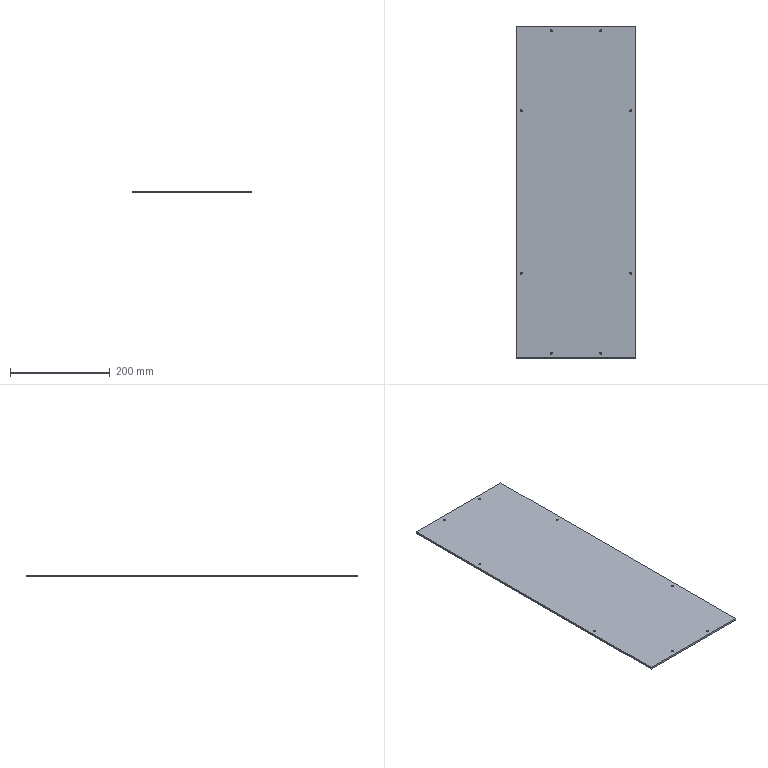Part | SolidWorks | features HoleWzd 2, MirrorPattern 2, Extrusion 1 | 1 solid | 22 faces | box 240 x 666 x 4 mm | volume 638958 mm3 | cylinder 16 | plane 6 | commonest cylinder face diameters 4 x16
STEP:
#1=CARTESIAN_POINT('',(-108.,163.,2.));
#2=VERTEX_POINT('',#1);
#3=CARTESIAN_POINT('',(-112.,163.,2.));
#4=VERTEX_POINT('',#3);
#5=CARTESIAN_POINT('',(-110.,163.,2.));
#6=DIRECTION('',(0.,0.,-1.));
#7=DIRECTION('',(-1.,0.,0.));
#8=AXIS2_PLACEMENT_3D('',#5,#6,#7);
#9=CIRCLE('',#8,2.);
#10=EDGE_CURVE('',#2,#4,#9,.T.);
#11=ORIENTED_EDGE('',*,*,#10,.F.);
#12=CARTESIAN_POINT('',(-108.,163.,-2.));
#13=VERTEX_POINT('',#12);
#14=CARTESIAN_POINT('',(-108.,163.,-2.));
#15=DIRECTION('',(0.,0.,-1.));
#16=VECTOR('',#15,1000.);
#17=LINE('',#14,#16);
#18=EDGE_CURVE('',#2,#13,#17,.T.);
#19=ORIENTED_EDGE('',*,*,#18,.T.);
#20=CARTESIAN_POINT('',(-112.,163.,-2.));
#21=VERTEX_POINT('',#20);
#22=CARTESIAN_POINT('',(-110.,163.,-2.));
#23=DIRECTION('',(0.,0.,-1.));
#24=DIRECTION('',(-1.,0.,0.));
#25=AXIS2_PLACEMENT_3D('',#22,#23,#24);
#26=CIRCLE('',#25,2.);
#27=EDGE_CURVE('',#13,#21,#26,.T.);
#28=ORIENTED_EDGE('',*,*,#27,.T.);
#29=CARTESIAN_POINT('',(-112.,163.,-2.));
#30=DIRECTION('',(0.,0.,-1.));
#31=VECTOR('',#30,1000.);
#32=LINE('',#29,#31);
#33=EDGE_CURVE('',#4,#21,#32,.T.);
#34=ORIENTED_EDGE('',*,*,#33,.F.);
#35=EDGE_LOOP('',(#11,#19,#28,#34));
#36=FACE_OUTER_BOUND('',#35,.T.);
#37=CARTESIAN_POINT('',(-110.,163.,-2.));
#38=DIRECTION('',(0.,0.,-1.));
#39=DIRECTION('',(-1.,0.,0.));
#40=AXIS2_PLACEMENT_3D('',#37,#38,#39);
#41=CYLINDRICAL_SURFACE('',#40,2.);
#42=ADVANCED_FACE('',(#36),#41,.F.);
#43=CARTESIAN_POINT('',(-108.,-163.,2.));
#44=VERTEX_POINT('',#43);
#45=CARTESIAN_POINT('',(-112.,-163.,2.));
#46=VERTEX_POINT('',#45);
#47=CARTESIAN_POINT('',(-110.,-163.,2.));
#48=DIRECTION('',(0.,0.,-1.));
#49=DIRECTION('',(-1.,0.,0.));
#50=AXIS2_PLACEMENT_3D('',#47,#48,#49);
#51=CIRCLE('',#50,2.);
#52=EDGE_CURVE('',#44,#46,#51,.T.);
#53=ORIENTED_EDGE('',*,*,#52,.F.);
#54=CARTESIAN_POINT('',(-108.,-163.,-2.));
#55=VERTEX_POINT('',#54);
#56=CARTESIAN_POINT('',(-108.,-163.,-2.));
#57=DIRECTION('',(0.,0.,-1.));
#58=VECTOR('',#57,1000.);
#59=LINE('',#56,#58);
#60=EDGE_CURVE('',#44,#55,#59,.T.);
#61=ORIENTED_EDGE('',*,*,#60,.T.);
#62=CARTESIAN_POINT('',(-112.,-163.,-2.));
#63=VERTEX_POINT('',#62);
#64=CARTESIAN_POINT('',(-110.,-163.,-2.));
#65=DIRECTION('',(0.,0.,-1.));
#66=DIRECTION('',(-1.,0.,0.));
#67=AXIS2_PLACEMENT_3D('',#64,#65,#66);
#68=CIRCLE('',#67,2.);
#69=EDGE_CURVE('',#55,#63,#68,.T.);
#70=ORIENTED_EDGE('',*,*,#69,.T.);
#71=CARTESIAN_POINT('',(-112.,-163.,-2.));
#72=DIRECTION('',(0.,0.,-1.));
#73=VECTOR('',#72,1000.);
#74=LINE('',#71,#73);
#75=EDGE_CURVE('',#46,#63,#74,.T.);
#76=ORIENTED_EDGE('',*,*,#75,.F.);
#77=EDGE_LOOP('',(#53,#61,#70,#76));
#78=FACE_OUTER_BOUND('',#77,.T.);
#79=CARTESIAN_POINT('',(-110.,-163.,-2.));
#80=DIRECTION('',(0.,0.,-1.));
#81=DIRECTION('',(-1.,0.,0.));
#82=AXIS2_PLACEMENT_3D('',#79,#80,#81);
#83=CYLINDRICAL_SURFACE('',#82,2.);
#84=ADVANCED_FACE('',(#78),#83,.F.);
#85=CARTESIAN_POINT('',(52.,-323.,2.));
#86=VERTEX_POINT('',#85);
#87=CARTESIAN_POINT('',(48.,-323.,2.));
#88=VERTEX_POINT('',#87);
#89=CARTESIAN_POINT('',(50.,-323.,2.));
#90=DIRECTION('',(0.,0.,-1.));
#91=DIRECTION('',(-1.,0.,0.));
#92=AXIS2_PLACEMENT_3D('',#89,#90,#91);
#93=CIRCLE('',#92,2.);
#94=EDGE_CURVE('',#86,#88,#93,.T.);
#95=ORIENTED_EDGE('',*,*,#94,.F.);
#96=CARTESIAN_POINT('',(52.,-323.,-2.));
#97=VERTEX_POINT('',#96);
#98=CARTESIAN_POINT('',(52.,-323.,-2.));
#99=DIRECTION('',(0.,0.,-1.));
#100=VECTOR('',#99,1000.);
#101=LINE('',#98,#100);
#102=EDGE_CURVE('',#86,#97,#101,.T.);
#103=ORIENTED_EDGE('',*,*,#102,.T.);
#104=CARTESIAN_POINT('',(48.,-323.,-2.));
#105=VERTEX_POINT('',#104);
#106=CARTESIAN_POINT('',(50.,-323.,-2.));
#107=DIRECTION('',(0.,0.,-1.));
#108=DIRECTION('',(-1.,0.,0.));
#109=AXIS2_PLACEMENT_3D('',#106,#107,#108);
#110=CIRCLE('',#109,2.);
#111=EDGE_CURVE('',#97,#105,#110,.T.);
#112=ORIENTED_EDGE('',*,*,#111,.T.);
#113=CARTESIAN_POINT('',(48.,-323.,-2.));
#114=DIRECTION('',(0.,0.,-1.));
#115=VECTOR('',#114,1000.);
#116=LINE('',#113,#115);
#117=EDGE_CURVE('',#88,#105,#116,.T.);
#118=ORIENTED_EDGE('',*,*,#117,.F.);
#119=EDGE_LOOP('',(#95,#103,#112,#118));
#120=FACE_OUTER_BOUND('',#119,.T.);
#121=CARTESIAN_POINT('',(50.,-323.,-2.));
#122=DIRECTION('',(0.,0.,-1.));
#123=DIRECTION('',(-1.,0.,0.));
#124=AXIS2_PLACEMENT_3D('',#121,#122,#123);
#125=CYLINDRICAL_SURFACE('',#124,2.);
#126=ADVANCED_FACE('',(#120),#125,.F.);
#127=CARTESIAN_POINT('',(-48.,-323.,2.));
#128=VERTEX_POINT('',#127);
#129=CARTESIAN_POINT('',(-52.,-323.,2.));
#130=VERTEX_POINT('',#129);
#131=CARTESIAN_POINT('',(-50.,-323.,2.));
#132=DIRECTION('',(0.,0.,-1.));
#133=DIRECTION('',(-1.,0.,0.));
#134=AXIS2_PLACEMENT_3D('',#131,#132,#133);
#135=CIRCLE('',#134,2.);
#136=EDGE_CURVE('',#128,#130,#135,.T.);
#137=ORIENTED_EDGE('',*,*,#136,.F.);
#138=CARTESIAN_POINT('',(-48.,-323.,-2.));
#139=VERTEX_POINT('',#138);
#140=CARTESIAN_POINT('',(-48.,-323.,-2.));
#141=DIRECTION('',(0.,0.,-1.));
#142=VECTOR('',#141,1000.);
#143=LINE('',#140,#142);
#144=EDGE_CURVE('',#128,#139,#143,.T.);
#145=ORIENTED_EDGE('',*,*,#144,.T.);
#146=CARTESIAN_POINT('',(-52.,-323.,-2.));
#147=VERTEX_POINT('',#146);
#148=CARTESIAN_POINT('',(-50.,-323.,-2.));
#149=DIRECTION('',(0.,0.,-1.));
#150=DIRECTION('',(-1.,0.,0.));
#151=AXIS2_PLACEMENT_3D('',#148,#149,#150);
#152=CIRCLE('',#151,2.);
#153=EDGE_CURVE('',#139,#147,#152,.T.);
#154=ORIENTED_EDGE('',*,*,#153,.T.);
#155=CARTESIAN_POINT('',(-52.,-323.,-2.));
#156=DIRECTION('',(0.,0.,-1.));
#157=VECTOR('',#156,1000.);
#158=LINE('',#155,#157);
#159=EDGE_CURVE('',#130,#147,#158,.T.);
#160=ORIENTED_EDGE('',*,*,#159,.F.);
#161=EDGE_LOOP('',(#137,#145,#154,#160));
#162=FACE_OUTER_BOUND('',#161,.T.);
#163=CARTESIAN_POINT('',(-50.,-323.,-2.));
#164=DIRECTION('',(0.,0.,-1.));
#165=DIRECTION('',(-1.,0.,0.));
#166=AXIS2_PLACEMENT_3D('',#163,#164,#165);
#167=CYLINDRICAL_SURFACE('',#166,2.);
#168=ADVANCED_FACE('',(#162),#167,.F.);
#169=CARTESIAN_POINT('',(52.,323.,2.));
#170=VERTEX_POINT('',#169);
#171=CARTESIAN_POINT('',(48.,323.,2.));
#172=VERTEX_POINT('',#171);
#173=CARTESIAN_POINT('',(50.,323.,2.));
#174=DIRECTION('',(0.,0.,-1.));
#175=DIRECTION('',(-1.,0.,0.));
#176=AXIS2_PLACEMENT_3D('',#173,#174,#175);
#177=CIRCLE('',#176,2.);
#178=EDGE_CURVE('',#170,#172,#177,.T.);
#179=ORIENTED_EDGE('',*,*,#178,.F.);
#180=CARTESIAN_POINT('',(52.,323.,-2.));
#181=VERTEX_POINT('',#180);
#182=CARTESIAN_POINT('',(52.,323.,-2.));
#183=DIRECTION('',(0.,0.,-1.));
#184=VECTOR('',#183,1000.);
#185=LINE('',#182,#184);
#186=EDGE_CURVE('',#170,#181,#185,.T.);
#187=ORIENTED_EDGE('',*,*,#186,.T.);
#188=CARTESIAN_POINT('',(48.,323.,-2.));
#189=VERTEX_POINT('',#188);
#190=CARTESIAN_POINT('',(50.,323.,-2.));
#191=DIRECTION('',(0.,0.,-1.));
#192=DIRECTION('',(-1.,0.,0.));
#193=AXIS2_PLACEMENT_3D('',#190,#191,#192);
#194=CIRCLE('',#193,2.);
#195=EDGE_CURVE('',#181,#189,#194,.T.);
#196=ORIENTED_EDGE('',*,*,#195,.T.);
#197=CARTESIAN_POINT('',(48.,323.,-2.));
#198=DIRECTION('',(0.,0.,-1.));
#199=VECTOR('',#198,1000.);
#200=LINE('',#197,#199);
#201=EDGE_CURVE('',#172,#189,#200,.T.);
#202=ORIENTED_EDGE('',*,*,#201,.F.);
#203=EDGE_LOOP('',(#179,#187,#196,#202));
#204=FACE_OUTER_BOUND('',#203,.T.);
#205=CARTESIAN_POINT('',(50.,323.,-2.));
#206=DIRECTION('',(0.,0.,-1.));
#207=DIRECTION('',(-1.,0.,0.));
#208=AXIS2_PLACEMENT_3D('',#205,#206,#207);
#209=CYLINDRICAL_SURFACE('',#208,2.);
#210=ADVANCED_FACE('',(#204),#209,.F.);
#211=CARTESIAN_POINT('',(-48.,323.,2.));
#212=VERTEX_POINT('',#211);
#213=CARTESIAN_POINT('',(-52.,323.,2.));
#214=VERTEX_POINT('',#213);
#215=CARTESIAN_POINT('',(-50.,323.,2.));
#216=DIRECTION('',(0.,0.,-1.));
#217=DIRECTION('',(-1.,0.,0.));
#218=AXIS2_PLACEMENT_3D('',#215,#216,#217);
#219=CIRCLE('',#218,2.);
#220=EDGE_CURVE('',#212,#214,#219,.T.);
#221=ORIENTED_EDGE('',*,*,#220,.F.);
#222=CARTESIAN_POINT('',(-48.,323.,-2.));
#223=VERTEX_POINT('',#222);
#224=CARTESIAN_POINT('',(-48.,323.,-2.));
#225=DIRECTION('',(0.,0.,-1.));
#226=VECTOR('',#225,1000.);
#227=LINE('',#224,#226);
#228=EDGE_CURVE('',#212,#223,#227,.T.);
#229=ORIENTED_EDGE('',*,*,#228,.T.);
#230=CARTESIAN_POINT('',(-52.,323.,-2.));
#231=VERTEX_POINT('',#230);
#232=CARTESIAN_POINT('',(-50.,323.,-2.));
#233=DIRECTION('',(0.,0.,-1.));
#234=DIRECTION('',(-1.,0.,0.));
#235=AXIS2_PLACEMENT_3D('',#232,#233,#234);
#236=CIRCLE('',#235,2.);
#237=EDGE_CURVE('',#223,#231,#236,.T.);
#238=ORIENTED_EDGE('',*,*,#237,.T.);
#239=CARTESIAN_POINT('',(-52.,323.,-2.));
#240=DIRECTION('',(0.,0.,-1.));
#241=VECTOR('',#240,1000.);
#242=LINE('',#239,#241);
#243=EDGE_CURVE('',#214,#231,#242,.T.);
#244=ORIENTED_EDGE('',*,*,#243,.F.);
#245=EDGE_LOOP('',(#221,#229,#238,#244));
#246=FACE_OUTER_BOUND('',#245,.T.);
#247=CARTESIAN_POINT('',(-50.,323.,-2.));
#248=DIRECTION('',(0.,0.,-1.));
#249=DIRECTION('',(-1.,0.,0.));
#250=AXIS2_PLACEMENT_3D('',#247,#248,#249);
#251=CYLINDRICAL_SURFACE('',#250,2.);
#252=ADVANCED_FACE('',(#246),#251,.F.);
#253=CARTESIAN_POINT('',(112.,163.,2.));
#254=VERTEX_POINT('',#253);
#255=CARTESIAN_POINT('',(108.,163.,2.));
#256=VERTEX_POINT('',#255);
#257=CARTESIAN_POINT('',(110.,163.,2.));
#258=DIRECTION('',(0.,0.,-1.));
#259=DIRECTION('',(-1.,0.,0.));
#260=AXIS2_PLACEMENT_3D('',#257,#258,#259);
#261=CIRCLE('',#260,2.);
#262=EDGE_CURVE('',#254,#256,#261,.T.);
#263=ORIENTED_EDGE('',*,*,#262,.F.);
#264=CARTESIAN_POINT('',(112.,163.,-2.));
#265=VERTEX_POINT('',#264);
#266=CARTESIAN_POINT('',(112.,163.,-2.));
#267=DIRECTION('',(0.,0.,-1.));
#268=VECTOR('',#267,1000.);
#269=LINE('',#266,#268);
#270=EDGE_CURVE('',#254,#265,#269,.T.);
#271=ORIENTED_EDGE('',*,*,#270,.T.);
#272=CARTESIAN_POINT('',(108.,163.,-2.));
#273=VERTEX_POINT('',#272);
#274=CARTESIAN_POINT('',(110.,163.,-2.));
#275=DIRECTION('',(0.,0.,-1.));
#276=DIRECTION('',(-1.,0.,0.));
#277=AXIS2_PLACEMENT_3D('',#274,#275,#276);
#278=CIRCLE('',#277,2.);
#279=EDGE_CURVE('',#265,#273,#278,.T.);
#280=ORIENTED_EDGE('',*,*,#279,.T.);
#281=CARTESIAN_POINT('',(108.,163.,-2.));
#282=DIRECTION('',(0.,0.,-1.));
#283=VECTOR('',#282,1000.);
#284=LINE('',#281,#283);
#285=EDGE_CURVE('',#256,#273,#284,.T.);
#286=ORIENTED_EDGE('',*,*,#285,.F.);
#287=EDGE_LOOP('',(#263,#271,#280,#286));
#288=FACE_OUTER_BOUND('',#287,.T.);
#289=CARTESIAN_POINT('',(110.,163.,-2.));
#290=DIRECTION('',(0.,0.,-1.));
#291=DIRECTION('',(-1.,0.,0.));
#292=AXIS2_PLACEMENT_3D('',#289,#290,#291);
#293=CYLINDRICAL_SURFACE('',#292,2.);
#294=ADVANCED_FACE('',(#288),#293,.F.);
#295=CARTESIAN_POINT('',(112.,-163.,2.));
#296=VERTEX_POINT('',#295);
#297=CARTESIAN_POINT('',(108.,-163.,2.));
#298=VERTEX_POINT('',#297);
#299=CARTESIAN_POINT('',(110.,-163.,2.));
#300=DIRECTION('',(0.,0.,-1.));
#301=DIRECTION('',(-1.,0.,0.));
#302=AXIS2_PLACEMENT_3D('',#299,#300,#301);
#303=CIRCLE('',#302,2.);
#304=EDGE_CURVE('',#296,#298,#303,.T.);
#305=ORIENTED_EDGE('',*,*,#304,.F.);
#306=CARTESIAN_POINT('',(112.,-163.,-2.));
#307=VERTEX_POINT('',#306);
#308=CARTESIAN_POINT('',(112.,-163.,-2.));
#309=DIRECTION('',(0.,0.,-1.));
#310=VECTOR('',#309,1000.);
#311=LINE('',#308,#310);
#312=EDGE_CURVE('',#296,#307,#311,.T.);
#313=ORIENTED_EDGE('',*,*,#312,.T.);
#314=CARTESIAN_POINT('',(108.,-163.,-2.));
#315=VERTEX_POINT('',#314);
#316=CARTESIAN_POINT('',(110.,-163.,-2.));
#317=DIRECTION('',(0.,0.,-1.));
#318=DIRECTION('',(-1.,0.,0.));
#319=AXIS2_PLACEMENT_3D('',#316,#317,#318);
#320=CIRCLE('',#319,2.);
#321=EDGE_CURVE('',#307,#315,#320,.T.);
#322=ORIENTED_EDGE('',*,*,#321,.T.);
#323=CARTESIAN_POINT('',(108.,-163.,-2.));
#324=DIRECTION('',(0.,0.,-1.));
#325=VECTOR('',#324,1000.);
#326=LINE('',#323,#325);
#327=EDGE_CURVE('',#298,#315,#326,.T.);
#328=ORIENTED_EDGE('',*,*,#327,.F.);
#329=EDGE_LOOP('',(#305,#313,#322,#328));
#330=FACE_OUTER_BOUND('',#329,.T.);
#331=CARTESIAN_POINT('',(110.,-163.,-2.));
#332=DIRECTION('',(0.,0.,-1.));
#333=DIRECTION('',(-1.,0.,0.));
#334=AXIS2_PLACEMENT_3D('',#331,#332,#333);
#335=CYLINDRICAL_SURFACE('',#334,2.);
#336=ADVANCED_FACE('',(#330),#335,.F.);
#337=CARTESIAN_POINT('',(120.,-333.,-2.));
#338=VERTEX_POINT('',#337);
#339=CARTESIAN_POINT('',(120.,333.,-2.));
#340=VERTEX_POINT('',#339);
#341=CARTESIAN_POINT('',(120.,-333.,-2.));
#342=DIRECTION('',(0.,1.,0.));
#343=VECTOR('',#342,1000.);
#344=LINE('',#341,#343);
#345=EDGE_CURVE('',#338,#340,#344,.T.);
#346=ORIENTED_EDGE('',*,*,#345,.T.);
#347=CARTESIAN_POINT('',(120.,333.,2.));
#348=VERTEX_POINT('',#347);
#349=CARTESIAN_POINT('',(120.,333.,2.));
#350=DIRECTION('',(0.,0.,-1.));
#351=VECTOR('',#350,1000.);
#352=LINE('',#349,#351);
#353=EDGE_CURVE('',#348,#340,#352,.T.);
#354=ORIENTED_EDGE('',*,*,#353,.F.);
#355=CARTESIAN_POINT('',(120.,-333.,2.));
#356=VERTEX_POINT('',#355);
#357=CARTESIAN_POINT('',(120.,-333.,2.));
#358=DIRECTION('',(0.,1.,0.));
#359=VECTOR('',#358,1000.);
#360=LINE('',#357,#359);
#361=EDGE_CURVE('',#356,#348,#360,.T.);
#362=ORIENTED_EDGE('',*,*,#361,.F.);
#363=CARTESIAN_POINT('',(120.,-333.,2.));
#364=DIRECTION('',(0.,0.,-1.));
#365=VECTOR('',#364,1000.);
#366=LINE('',#363,#365);
#367=EDGE_CURVE('',#356,#338,#366,.T.);
#368=ORIENTED_EDGE('',*,*,#367,.T.);
#369=EDGE_LOOP('',(#346,#354,#362,#368));
#370=FACE_OUTER_BOUND('',#369,.T.);
#371=CARTESIAN_POINT('',(120.,-333.,2.));
#372=DIRECTION('',(-1.,0.,0.));
#373=DIRECTION('',(0.,0.,1.));
#374=AXIS2_PLACEMENT_3D('',#371,#372,#373);
#375=PLANE('',#374);
#376=ADVANCED_FACE('',(#370),#375,.F.);
#377=CARTESIAN_POINT('',(-120.,333.,-2.));
#378=VERTEX_POINT('',#377);
#379=CARTESIAN_POINT('',(-120.,333.,-2.));
#380=DIRECTION('',(-1.,0.,0.));
#381=VECTOR('',#380,1000.);
#382=LINE('',#379,#381);
#383=EDGE_CURVE('',#340,#378,#382,.T.);
#384=ORIENTED_EDGE('',*,*,#383,.T.);
#385=CARTESIAN_POINT('',(-120.,333.,2.));
#386=VERTEX_POINT('',#385);
#387=CARTESIAN_POINT('',(-120.,333.,2.));
#388=DIRECTION('',(0.,0.,-1.));
#389=VECTOR('',#388,1000.);
#390=LINE('',#387,#389);
#391=EDGE_CURVE('',#386,#378,#390,.T.);
#392=ORIENTED_EDGE('',*,*,#391,.F.);
#393=CARTESIAN_POINT('',(-120.,333.,2.));
#394=DIRECTION('',(-1.,0.,0.));
#395=VECTOR('',#394,1000.);
#396=LINE('',#393,#395);
#397=EDGE_CURVE('',#348,#386,#396,.T.);
#398=ORIENTED_EDGE('',*,*,#397,.F.);
#399=ORIENTED_EDGE('',*,*,#353,.T.);
#400=EDGE_LOOP('',(#384,#392,#398,#399));
#401=FACE_OUTER_BOUND('',#400,.T.);
#402=CARTESIAN_POINT('',(-120.,333.,2.));
#403=DIRECTION('',(0.,-1.,0.));
#404=DIRECTION('',(0.,0.,-1.));
#405=AXIS2_PLACEMENT_3D('',#402,#403,#404);
#406=PLANE('',#405);
#407=ADVANCED_FACE('',(#401),#406,.F.);
#408=CARTESIAN_POINT('',(-120.,-333.,-2.));
#409=VERTEX_POINT('',#408);
#410=CARTESIAN_POINT('',(-120.,-333.,-2.));
#411=DIRECTION('',(0.,-1.,0.));
#412=VECTOR('',#411,1000.);
#413=LINE('',#410,#412);
#414=EDGE_CURVE('',#378,#409,#413,.T.);
#415=ORIENTED_EDGE('',*,*,#414,.T.);
#416=CARTESIAN_POINT('',(-120.,-333.,2.));
#417=VERTEX_POINT('',#416);
#418=CARTESIAN_POINT('',(-120.,-333.,2.));
#419=DIRECTION('',(0.,0.,-1.));
#420=VECTOR('',#419,1000.);
#421=LINE('',#418,#420);
#422=EDGE_CURVE('',#417,#409,#421,.T.);
#423=ORIENTED_EDGE('',*,*,#422,.F.);
#424=CARTESIAN_POINT('',(-120.,-333.,2.));
#425=DIRECTION('',(0.,-1.,0.));
#426=VECTOR('',#425,1000.);
#427=LINE('',#424,#426);
#428=EDGE_CURVE('',#386,#417,#427,.T.);
#429=ORIENTED_EDGE('',*,*,#428,.F.);
#430=ORIENTED_EDGE('',*,*,#391,.T.);
#431=EDGE_LOOP('',(#415,#423,#429,#430));
#432=FACE_OUTER_BOUND('',#431,.T.);
#433=CARTESIAN_POINT('',(-120.,-333.,2.));
#434=DIRECTION('',(1.,0.,0.));
#435=DIRECTION('',(0.,0.,-1.));
#436=AXIS2_PLACEMENT_3D('',#433,#434,#435);
#437=PLANE('',#436);
#438=ADVANCED_FACE('',(#432),#437,.F.);
#439=CARTESIAN_POINT('',(-120.,-333.,-2.));
#440=DIRECTION('',(1.,0.,0.));
#441=VECTOR('',#440,1000.);
#442=LINE('',#439,#441);
#443=EDGE_CURVE('',#409,#338,#442,.T.);
#444=ORIENTED_EDGE('',*,*,#443,.T.);
#445=ORIENTED_EDGE('',*,*,#367,.F.);
#446=CARTESIAN_POINT('',(-120.,-333.,2.));
#447=DIRECTION('',(1.,0.,0.));
#448=VECTOR('',#447,1000.);
#449=LINE('',#446,#448);
#450=EDGE_CURVE('',#417,#356,#449,.T.);
#451=ORIENTED_EDGE('',*,*,#450,.F.);
#452=ORIENTED_EDGE('',*,*,#422,.T.);
#453=EDGE_LOOP('',(#444,#445,#451,#452));
#454=FACE_OUTER_BOUND('',#453,.T.);
#455=CARTESIAN_POINT('',(-120.,-333.,2.));
#456=DIRECTION('',(0.,1.,0.));
#457=DIRECTION('',(0.,0.,1.));
#458=AXIS2_PLACEMENT_3D('',#455,#456,#457);
#459=PLANE('',#458);
#460=ADVANCED_FACE('',(#454),#459,.F.);
#461=CARTESIAN_POINT('',(-110.,163.,2.));
#462=DIRECTION('',(0.,0.,-1.));
#463=DIRECTION('',(-1.,0.,0.));
#464=AXIS2_PLACEMENT_3D('',#461,#462,#463);
#465=CIRCLE('',#464,2.);
#466=EDGE_CURVE('',#4,#2,#465,.T.);
#467=ORIENTED_EDGE('',*,*,#466,.T.);
#468=ORIENTED_EDGE('',*,*,#10,.T.);
#469=EDGE_LOOP('',(#467,#468));
#470=FACE_BOUND('',#469,.T.);
#471=CARTESIAN_POINT('',(-110.,-163.,2.));
#472=DIRECTION('',(0.,0.,-1.));
#473=DIRECTION('',(-1.,0.,0.));
#474=AXIS2_PLACEMENT_3D('',#471,#472,#473);
#475=CIRCLE('',#474,2.);
#476=EDGE_CURVE('',#46,#44,#475,.T.);
#477=ORIENTED_EDGE('',*,*,#476,.T.);
#478=ORIENTED_EDGE('',*,*,#52,.T.);
#479=EDGE_LOOP('',(#477,#478));
#480=FACE_BOUND('',#479,.T.);
#481=CARTESIAN_POINT('',(50.,-323.,2.));
#482=DIRECTION('',(0.,0.,-1.));
#483=DIRECTION('',(-1.,0.,0.));
#484=AXIS2_PLACEMENT_3D('',#481,#482,#483);
#485=CIRCLE('',#484,2.);
#486=EDGE_CURVE('',#88,#86,#485,.T.);
#487=ORIENTED_EDGE('',*,*,#486,.T.);
#488=ORIENTED_EDGE('',*,*,#94,.T.);
#489=EDGE_LOOP('',(#487,#488));
#490=FACE_BOUND('',#489,.T.);
#491=CARTESIAN_POINT('',(-50.,-323.,2.));
#492=DIRECTION('',(0.,0.,-1.));
#493=DIRECTION('',(-1.,0.,0.));
#494=AXIS2_PLACEMENT_3D('',#491,#492,#493);
#495=CIRCLE('',#494,2.);
#496=EDGE_CURVE('',#130,#128,#495,.T.);
#497=ORIENTED_EDGE('',*,*,#496,.T.);
#498=ORIENTED_EDGE('',*,*,#136,.T.);
#499=EDGE_LOOP('',(#497,#498));
#500=FACE_BOUND('',#499,.T.);
#501=CARTESIAN_POINT('',(50.,323.,2.));
#502=DIRECTION('',(0.,0.,-1.));
#503=DIRECTION('',(-1.,0.,0.));
#504=AXIS2_PLACEMENT_3D('',#501,#502,#503);
#505=CIRCLE('',#504,2.);
#506=EDGE_CURVE('',#172,#170,#505,.T.);
#507=ORIENTED_EDGE('',*,*,#506,.T.);
#508=ORIENTED_EDGE('',*,*,#178,.T.);
#509=EDGE_LOOP('',(#507,#508));
#510=FACE_BOUND('',#509,.T.);
#511=CARTESIAN_POINT('',(-50.,323.,2.));
#512=DIRECTION('',(0.,0.,-1.));
#513=DIRECTION('',(-1.,0.,0.));
#514=AXIS2_PLACEMENT_3D('',#511,#512,#513);
#515=CIRCLE('',#514,2.);
#516=EDGE_CURVE('',#214,#212,#515,.T.);
#517=ORIENTED_EDGE('',*,*,#516,.T.);
#518=ORIENTED_EDGE('',*,*,#220,.T.);
#519=EDGE_LOOP('',(#517,#518));
#520=FACE_BOUND('',#519,.T.);
#521=CARTESIAN_POINT('',(110.,163.,2.));
#522=DIRECTION('',(0.,0.,-1.));
#523=DIRECTION('',(-1.,0.,0.));
#524=AXIS2_PLACEMENT_3D('',#521,#522,#523);
#525=CIRCLE('',#524,2.);
#526=EDGE_CURVE('',#256,#254,#525,.T.);
#527=ORIENTED_EDGE('',*,*,#526,.T.);
#528=ORIENTED_EDGE('',*,*,#262,.T.);
#529=EDGE_LOOP('',(#527,#528));
#530=FACE_BOUND('',#529,.T.);
#531=CARTESIAN_POINT('',(110.,-163.,2.));
#532=DIRECTION('',(0.,0.,-1.));
#533=DIRECTION('',(-1.,0.,0.));
#534=AXIS2_PLACEMENT_3D('',#531,#532,#533);
#535=CIRCLE('',#534,2.);
#536=EDGE_CURVE('',#298,#296,#535,.T.);
#537=ORIENTED_EDGE('',*,*,#536,.T.);
#538=ORIENTED_EDGE('',*,*,#304,.T.);
#539=EDGE_LOOP('',(#537,#538));
#540=FACE_BOUND('',#539,.T.);
#541=ORIENTED_EDGE('',*,*,#361,.T.);
#542=ORIENTED_EDGE('',*,*,#397,.T.);
#543=ORIENTED_EDGE('',*,*,#428,.T.);
#544=ORIENTED_EDGE('',*,*,#450,.T.);
#545=EDGE_LOOP('',(#541,#542,#543,#544));
#546=FACE_OUTER_BOUND('',#545,.T.);
#547=CARTESIAN_POINT('',(0.,0.,2.));
#548=DIRECTION('',(0.,0.,-1.));
#549=DIRECTION('',(-1.,0.,0.));
#550=AXIS2_PLACEMENT_3D('',#547,#548,#549);
#551=PLANE('',#550);
#552=ADVANCED_FACE('',(#470,#480,#490,#500,#510,#520,#530,#540,#546),#551,.F.);
#553=CARTESIAN_POINT('',(-110.,163.,-2.));
#554=DIRECTION('',(0.,0.,-1.));
#555=DIRECTION('',(-1.,0.,0.));
#556=AXIS2_PLACEMENT_3D('',#553,#554,#555);
#557=CIRCLE('',#556,2.);
#558=EDGE_CURVE('',#21,#13,#557,.T.);
#559=ORIENTED_EDGE('',*,*,#558,.F.);
#560=ORIENTED_EDGE('',*,*,#27,.F.);
#561=EDGE_LOOP('',(#559,#560));
#562=FACE_BOUND('',#561,.T.);
#563=CARTESIAN_POINT('',(-110.,-163.,-2.));
#564=DIRECTION('',(0.,0.,-1.));
#565=DIRECTION('',(-1.,0.,0.));
#566=AXIS2_PLACEMENT_3D('',#563,#564,#565);
#567=CIRCLE('',#566,2.);
#568=EDGE_CURVE('',#63,#55,#567,.T.);
#569=ORIENTED_EDGE('',*,*,#568,.F.);
#570=ORIENTED_EDGE('',*,*,#69,.F.);
#571=EDGE_LOOP('',(#569,#570));
#572=FACE_BOUND('',#571,.T.);
#573=CARTESIAN_POINT('',(50.,-323.,-2.));
#574=DIRECTION('',(0.,0.,-1.));
#575=DIRECTION('',(-1.,0.,0.));
#576=AXIS2_PLACEMENT_3D('',#573,#574,#575);
#577=CIRCLE('',#576,2.);
#578=EDGE_CURVE('',#105,#97,#577,.T.);
#579=ORIENTED_EDGE('',*,*,#578,.F.);
#580=ORIENTED_EDGE('',*,*,#111,.F.);
#581=EDGE_LOOP('',(#579,#580));
#582=FACE_BOUND('',#581,.T.);
#583=CARTESIAN_POINT('',(-50.,-323.,-2.));
#584=DIRECTION('',(0.,0.,-1.));
#585=DIRECTION('',(-1.,0.,0.));
#586=AXIS2_PLACEMENT_3D('',#583,#584,#585);
#587=CIRCLE('',#586,2.);
#588=EDGE_CURVE('',#147,#139,#587,.T.);
#589=ORIENTED_EDGE('',*,*,#588,.F.);
#590=ORIENTED_EDGE('',*,*,#153,.F.);
#591=EDGE_LOOP('',(#589,#590));
#592=FACE_BOUND('',#591,.T.);
#593=CARTESIAN_POINT('',(50.,323.,-2.));
#594=DIRECTION('',(0.,0.,-1.));
#595=DIRECTION('',(-1.,0.,0.));
#596=AXIS2_PLACEMENT_3D('',#593,#594,#595);
#597=CIRCLE('',#596,2.);
#598=EDGE_CURVE('',#189,#181,#597,.T.);
#599=ORIENTED_EDGE('',*,*,#598,.F.);
#600=ORIENTED_EDGE('',*,*,#195,.F.);
#601=EDGE_LOOP('',(#599,#600));
#602=FACE_BOUND('',#601,.T.);
#603=CARTESIAN_POINT('',(-50.,323.,-2.));
#604=DIRECTION('',(0.,0.,-1.));
#605=DIRECTION('',(-1.,0.,0.));
#606=AXIS2_PLACEMENT_3D('',#603,#604,#605);
#607=CIRCLE('',#606,2.);
#608=EDGE_CURVE('',#231,#223,#607,.T.);
#609=ORIENTED_EDGE('',*,*,#608,.F.);
#610=ORIENTED_EDGE('',*,*,#237,.F.);
#611=EDGE_LOOP('',(#609,#610));
#612=FACE_BOUND('',#611,.T.);
#613=CARTESIAN_POINT('',(110.,163.,-2.));
#614=DIRECTION('',(0.,0.,-1.));
#615=DIRECTION('',(-1.,0.,0.));
#616=AXIS2_PLACEMENT_3D('',#613,#614,#615);
#617=CIRCLE('',#616,2.);
#618=EDGE_CURVE('',#273,#265,#617,.T.);
#619=ORIENTED_EDGE('',*,*,#618,.F.);
#620=ORIENTED_EDGE('',*,*,#279,.F.);
#621=EDGE_LOOP('',(#619,#620));
#622=FACE_BOUND('',#621,.T.);
#623=CARTESIAN_POINT('',(110.,-163.,-2.));
#624=DIRECTION('',(0.,0.,-1.));
#625=DIRECTION('',(-1.,0.,0.));
#626=AXIS2_PLACEMENT_3D('',#623,#624,#625);
#627=CIRCLE('',#626,2.);
#628=EDGE_CURVE('',#315,#307,#627,.T.);
#629=ORIENTED_EDGE('',*,*,#628,.F.);
#630=ORIENTED_EDGE('',*,*,#321,.F.);
#631=EDGE_LOOP('',(#629,#630));
#632=FACE_BOUND('',#631,.T.);
#633=ORIENTED_EDGE('',*,*,#345,.F.);
#634=ORIENTED_EDGE('',*,*,#443,.F.);
#635=ORIENTED_EDGE('',*,*,#414,.F.);
#636=ORIENTED_EDGE('',*,*,#383,.F.);
#637=EDGE_LOOP('',(#633,#634,#635,#636));
#638=FACE_OUTER_BOUND('',#637,.T.);
#639=CARTESIAN_POINT('',(0.,0.,-2.));
#640=DIRECTION('',(0.,0.,-1.));
#641=DIRECTION('',(-1.,0.,0.));
#642=AXIS2_PLACEMENT_3D('',#639,#640,#641);
#643=PLANE('',#642);
#644=ADVANCED_FACE('',(#562,#572,#582,#592,#602,#612,#622,#632,#638),#643,.T.);
#645=ORIENTED_EDGE('',*,*,#312,.F.);
#646=ORIENTED_EDGE('',*,*,#536,.F.);
#647=ORIENTED_EDGE('',*,*,#327,.T.);
#648=ORIENTED_EDGE('',*,*,#628,.T.);
#649=EDGE_LOOP('',(#645,#646,#647,#648));
#650=FACE_OUTER_BOUND('',#649,.T.);
#651=CARTESIAN_POINT('',(110.,-163.,-2.));
#652=DIRECTION('',(0.,0.,-1.));
#653=DIRECTION('',(-1.,0.,0.));
#654=AXIS2_PLACEMENT_3D('',#651,#652,#653);
#655=CYLINDRICAL_SURFACE('',#654,2.);
#656=ADVANCED_FACE('',(#650),#655,.F.);
#657=ORIENTED_EDGE('',*,*,#270,.F.);
#658=ORIENTED_EDGE('',*,*,#526,.F.);
#659=ORIENTED_EDGE('',*,*,#285,.T.);
#660=ORIENTED_EDGE('',*,*,#618,.T.);
#661=EDGE_LOOP('',(#657,#658,#659,#660));
#662=FACE_OUTER_BOUND('',#661,.T.);
#663=CARTESIAN_POINT('',(110.,163.,-2.));
#664=DIRECTION('',(0.,0.,-1.));
#665=DIRECTION('',(-1.,0.,0.));
#666=AXIS2_PLACEMENT_3D('',#663,#664,#665);
#667=CYLINDRICAL_SURFACE('',#666,2.);
#668=ADVANCED_FACE('',(#662),#667,.F.);
#669=ORIENTED_EDGE('',*,*,#228,.F.);
#670=ORIENTED_EDGE('',*,*,#516,.F.);
#671=ORIENTED_EDGE('',*,*,#243,.T.);
#672=ORIENTED_EDGE('',*,*,#608,.T.);
#673=EDGE_LOOP('',(#669,#670,#671,#672));
#674=FACE_OUTER_BOUND('',#673,.T.);
#675=CARTESIAN_POINT('',(-50.,323.,-2.));
#676=DIRECTION('',(0.,0.,-1.));
#677=DIRECTION('',(-1.,0.,0.));
#678=AXIS2_PLACEMENT_3D('',#675,#676,#677);
#679=CYLINDRICAL_SURFACE('',#678,2.);
#680=ADVANCED_FACE('',(#674),#679,.F.);
#681=ORIENTED_EDGE('',*,*,#186,.F.);
#682=ORIENTED_EDGE('',*,*,#506,.F.);
#683=ORIENTED_EDGE('',*,*,#201,.T.);
#684=ORIENTED_EDGE('',*,*,#598,.T.);
#685=EDGE_LOOP('',(#681,#682,#683,#684));
#686=FACE_OUTER_BOUND('',#685,.T.);
#687=CARTESIAN_POINT('',(50.,323.,-2.));
#688=DIRECTION('',(0.,0.,-1.));
#689=DIRECTION('',(-1.,0.,0.));
#690=AXIS2_PLACEMENT_3D('',#687,#688,#689);
#691=CYLINDRICAL_SURFACE('',#690,2.);
#692=ADVANCED_FACE('',(#686),#691,.F.);
#693=ORIENTED_EDGE('',*,*,#144,.F.);
#694=ORIENTED_EDGE('',*,*,#496,.F.);
#695=ORIENTED_EDGE('',*,*,#159,.T.);
#696=ORIENTED_EDGE('',*,*,#588,.T.);
#697=EDGE_LOOP('',(#693,#694,#695,#696));
#698=FACE_OUTER_BOUND('',#697,.T.);
#699=CARTESIAN_POINT('',(-50.,-323.,-2.));
#700=DIRECTION('',(0.,0.,-1.));
#701=DIRECTION('',(-1.,0.,0.));
#702=AXIS2_PLACEMENT_3D('',#699,#700,#701);
#703=CYLINDRICAL_SURFACE('',#702,2.);
#704=ADVANCED_FACE('',(#698),#703,.F.);
#705=ORIENTED_EDGE('',*,*,#102,.F.);
#706=ORIENTED_EDGE('',*,*,#486,.F.);
#707=ORIENTED_EDGE('',*,*,#117,.T.);
#708=ORIENTED_EDGE('',*,*,#578,.T.);
#709=EDGE_LOOP('',(#705,#706,#707,#708));
#710=FACE_OUTER_BOUND('',#709,.T.);
#711=CARTESIAN_POINT('',(50.,-323.,-2.));
#712=DIRECTION('',(0.,0.,-1.));
#713=DIRECTION('',(-1.,0.,0.));
#714=AXIS2_PLACEMENT_3D('',#711,#712,#713);
#715=CYLINDRICAL_SURFACE('',#714,2.);
#716=ADVANCED_FACE('',(#710),#715,.F.);
#717=ORIENTED_EDGE('',*,*,#60,.F.);
#718=ORIENTED_EDGE('',*,*,#476,.F.);
#719=ORIENTED_EDGE('',*,*,#75,.T.);
#720=ORIENTED_EDGE('',*,*,#568,.T.);
#721=EDGE_LOOP('',(#717,#718,#719,#720));
#722=FACE_OUTER_BOUND('',#721,.T.);
#723=CARTESIAN_POINT('',(-110.,-163.,-2.));
#724=DIRECTION('',(0.,0.,-1.));
#725=DIRECTION('',(-1.,0.,0.));
#726=AXIS2_PLACEMENT_3D('',#723,#724,#725);
#727=CYLINDRICAL_SURFACE('',#726,2.);
#728=ADVANCED_FACE('',(#722),#727,.F.);
#729=ORIENTED_EDGE('',*,*,#18,.F.);
#730=ORIENTED_EDGE('',*,*,#466,.F.);
#731=ORIENTED_EDGE('',*,*,#33,.T.);
#732=ORIENTED_EDGE('',*,*,#558,.T.);
#733=EDGE_LOOP('',(#729,#730,#731,#732));
#734=FACE_OUTER_BOUND('',#733,.T.);
#735=CARTESIAN_POINT('',(-110.,163.,-2.));
#736=DIRECTION('',(0.,0.,-1.));
#737=DIRECTION('',(-1.,0.,0.));
#738=AXIS2_PLACEMENT_3D('',#735,#736,#737);
#739=CYLINDRICAL_SURFACE('',#738,2.);
#740=ADVANCED_FACE('',(#734),#739,.F.);
#741=CLOSED_SHELL('',(#42,#84,#126,#168,#210,#252,#294,#336,#376,#407,#438,#460,#552,#644,#656,#668,#680,#692,#704,#716,#728,#740));
#742=MANIFOLD_SOLID_BREP('',#741);
#743=CARTESIAN_POINT('',(0.,0.,0.));
#744=DIRECTION('',(0.,0.,1.));
#745=DIRECTION('',(1.,0.,0.));
#746=AXIS2_PLACEMENT_3D('',#743,#744,#745);
#747=(LENGTH_UNIT()NAMED_UNIT(*)SI_UNIT(.MILLI.,.METRE.));
#748=UNCERTAINTY_MEASURE_WITH_UNIT(LENGTH_MEASURE(0.00001),#747,'','');
#749=(NAMED_UNIT(*)PLANE_ANGLE_UNIT()SI_UNIT($,.RADIAN.));
#750=(NAMED_UNIT(*)SI_UNIT($,.STERADIAN.)SOLID_ANGLE_UNIT());
#751=(GEOMETRIC_REPRESENTATION_CONTEXT(3)GLOBAL_UNCERTAINTY_ASSIGNED_CONTEXT((#748))GLOBAL_UNIT_ASSIGNED_CONTEXT((#747,#749,#750))REPRESENTATION_CONTEXT('',''));
#752=ADVANCED_BREP_SHAPE_REPRESENTATION('',(#742,#746),#751);